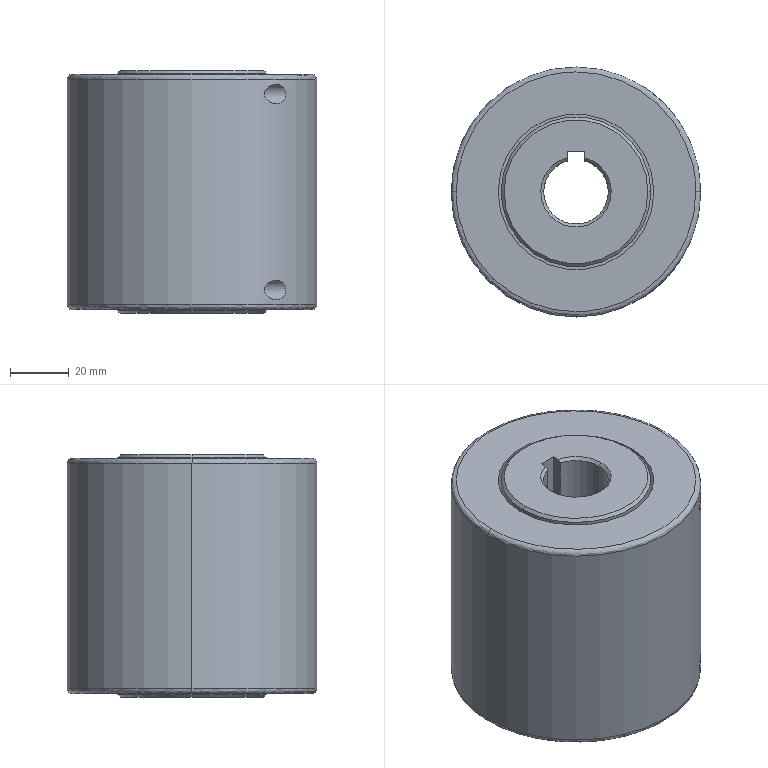Part | SolidWorks | features BaseBody 1 | 1 solid | 110 faces | box 85 x 85 x 82.7 mm | volume 299308 mm3 | plane 54 | cylinder 42 | cone 10 | spline 4 | commonest cylinder face diameters 4.667 x8 6.667 x8 51 x8 53 x8 22 x6 72.25 x2